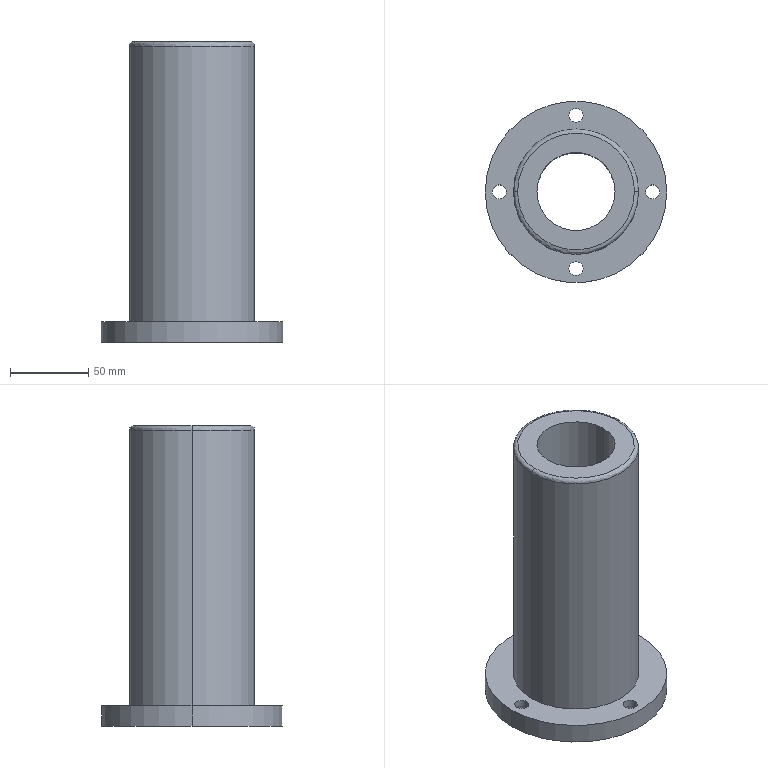Part | STEP file | LMG02-d50-Yiheda | 1 solid | 31 faces | box 116 x 116 x 192 mm | volume 653566 mm3 | cylinder 22 | plane 7 | spline 2 | commonest cylinder face diameters 9 x8 14 x8 50 x2 80 x2 116 x2
STEP:
#1=CARTESIAN_POINT('',(40.,0.,189.3));
#2=VERTEX_POINT('',#1);
#3=CARTESIAN_POINT('',(-40.,0.,189.3));
#4=VERTEX_POINT('',#3);
#5=CARTESIAN_POINT('',(0.,0.,189.3));
#6=DIRECTION('',(0.,0.,-1.));
#7=DIRECTION('',(-1.,0.,0.));
#8=AXIS2_PLACEMENT_3D('',#5,#6,#7);
#9=CIRCLE('',#8,40.);
#10=EDGE_CURVE('',#2,#4,#9,.T.);
#11=ORIENTED_EDGE('',*,*,#10,.F.);
#12=CARTESIAN_POINT('',(37.3,0.,192.));
#13=VERTEX_POINT('',#12);
#14=CARTESIAN_POINT('',(37.3,0.,189.3));
#15=DIRECTION('',(0.,-1.,0.));
#16=DIRECTION('',(1.,0.,0.));
#17=AXIS2_PLACEMENT_3D('',#14,#15,#16);
#18=CIRCLE('',#17,2.7);
#19=EDGE_CURVE('',#2,#13,#18,.T.);
#20=ORIENTED_EDGE('',*,*,#19,.T.);
#21=CARTESIAN_POINT('',(-37.3,0.,192.));
#22=VERTEX_POINT('',#21);
#23=CARTESIAN_POINT('',(37.3,0.,192.));
#24=CARTESIAN_POINT('',(37.3,-74.6,192.));
#25=CARTESIAN_POINT('',(-37.3,-74.6,192.));
#26=CARTESIAN_POINT('',(-37.3,0.,192.));
#27=(BOUNDED_CURVE()B_SPLINE_CURVE(3,(#23,#24,#25,#26),.UNSPECIFIED.,.F.,.T.)B_SPLINE_CURVE_WITH_KNOTS((4,4),(0.5,1.),.UNSPECIFIED.)CURVE()GEOMETRIC_REPRESENTATION_ITEM()RATIONAL_B_SPLINE_CURVE((1.,0.3333,0.3333,1.))REPRESENTATION_ITEM(''));
#28=EDGE_CURVE('',#13,#22,#27,.T.);
#29=ORIENTED_EDGE('',*,*,#28,.T.);
#30=CARTESIAN_POINT('',(-37.3,0.,189.3));
#31=DIRECTION('',(0.,1.,0.));
#32=DIRECTION('',(-1.,0.,0.));
#33=AXIS2_PLACEMENT_3D('',#30,#31,#32);
#34=CIRCLE('',#33,2.7);
#35=EDGE_CURVE('',#4,#22,#34,.T.);
#36=ORIENTED_EDGE('',*,*,#35,.F.);
#37=EDGE_LOOP('',(#11,#20,#29,#36));
#38=FACE_OUTER_BOUND('',#37,.T.);
#39=CARTESIAN_POINT('',(40.,0.,189.3));
#40=CARTESIAN_POINT('',(40.,-80.,189.3));
#41=CARTESIAN_POINT('',(-40.,-80.,189.3));
#42=CARTESIAN_POINT('',(-40.,0.,189.3));
#43=CARTESIAN_POINT('',(40.,0.,190.882));
#44=CARTESIAN_POINT('',(40.,-80.,190.882));
#45=CARTESIAN_POINT('',(-40.,-80.,190.882));
#46=CARTESIAN_POINT('',(-40.,0.,190.882));
#47=CARTESIAN_POINT('',(38.882,0.,192.));
#48=CARTESIAN_POINT('',(38.882,-77.763,192.));
#49=CARTESIAN_POINT('',(-38.882,-77.763,192.));
#50=CARTESIAN_POINT('',(-38.882,0.,192.));
#51=CARTESIAN_POINT('',(37.3,0.,192.));
#52=CARTESIAN_POINT('',(37.3,-74.6,192.));
#53=CARTESIAN_POINT('',(-37.3,-74.6,192.));
#54=CARTESIAN_POINT('',(-37.3,0.,192.));
#55=(BOUNDED_SURFACE()B_SPLINE_SURFACE(3,3,((#39,#40,#41,#42),(#43,#44,#45,#46),(#47,#48,#49,#50),(#51,#52,#53,#54)),.UNSPECIFIED.,.F.,.F.,.T.)B_SPLINE_SURFACE_WITH_KNOTS((4,4),(4,4),(0.,1.),(0.,1.),.UNSPECIFIED.)GEOMETRIC_REPRESENTATION_ITEM()RATIONAL_B_SPLINE_SURFACE(((1.,0.3333,0.3333,1.),(0.8047,0.2682,0.2682,0.8047),(0.8047,0.2682,0.2682,0.8047),(1.,0.3333,0.3333,1.)))REPRESENTATION_ITEM('')SURFACE());
#56=ADVANCED_FACE('',(#38),#55,.T.);
#57=CARTESIAN_POINT('',(0.,0.,189.3));
#58=DIRECTION('',(0.,0.,-1.));
#59=DIRECTION('',(-1.,0.,0.));
#60=AXIS2_PLACEMENT_3D('',#57,#58,#59);
#61=CIRCLE('',#60,40.);
#62=EDGE_CURVE('',#4,#2,#61,.T.);
#63=ORIENTED_EDGE('',*,*,#62,.T.);
#64=CARTESIAN_POINT('',(40.,0.,13.));
#65=VERTEX_POINT('',#64);
#66=CARTESIAN_POINT('',(40.,0.,0.));
#67=DIRECTION('',(0.,0.,-1.));
#68=VECTOR('',#67,1000.);
#69=LINE('',#66,#68);
#70=EDGE_CURVE('',#2,#65,#69,.T.);
#71=ORIENTED_EDGE('',*,*,#70,.T.);
#72=CARTESIAN_POINT('',(-40.,0.,13.));
#73=VERTEX_POINT('',#72);
#74=CARTESIAN_POINT('',(0.,0.,13.));
#75=DIRECTION('',(0.,0.,1.));
#76=DIRECTION('',(-1.,0.,0.));
#77=AXIS2_PLACEMENT_3D('',#74,#75,#76);
#78=CIRCLE('',#77,40.);
#79=EDGE_CURVE('',#65,#73,#78,.T.);
#80=ORIENTED_EDGE('',*,*,#79,.T.);
#81=CARTESIAN_POINT('',(-40.,0.,0.));
#82=DIRECTION('',(0.,0.,-1.));
#83=VECTOR('',#82,1000.);
#84=LINE('',#81,#83);
#85=EDGE_CURVE('',#4,#73,#84,.T.);
#86=ORIENTED_EDGE('',*,*,#85,.F.);
#87=EDGE_LOOP('',(#63,#71,#80,#86));
#88=FACE_OUTER_BOUND('',#87,.T.);
#89=CARTESIAN_POINT('',(0.,0.,0.));
#90=DIRECTION('',(0.,0.,-1.));
#91=DIRECTION('',(-1.,0.,0.));
#92=AXIS2_PLACEMENT_3D('',#89,#90,#91);
#93=CYLINDRICAL_SURFACE('',#92,40.);
#94=ADVANCED_FACE('',(#88),#93,.T.);
#95=CARTESIAN_POINT('',(58.,0.,13.));
#96=VERTEX_POINT('',#95);
#97=CARTESIAN_POINT('',(-58.,0.,13.));
#98=VERTEX_POINT('',#97);
#99=CARTESIAN_POINT('',(0.,0.,13.));
#100=DIRECTION('',(0.,0.,1.));
#101=DIRECTION('',(-1.,0.,0.));
#102=AXIS2_PLACEMENT_3D('',#99,#100,#101);
#103=CIRCLE('',#102,58.);
#104=EDGE_CURVE('',#96,#98,#103,.T.);
#105=ORIENTED_EDGE('',*,*,#104,.F.);
#106=CARTESIAN_POINT('',(58.,0.,0.));
#107=VERTEX_POINT('',#106);
#108=CARTESIAN_POINT('',(58.,0.,13.));
#109=DIRECTION('',(0.,0.,-1.));
#110=VECTOR('',#109,1000.);
#111=LINE('',#108,#110);
#112=EDGE_CURVE('',#96,#107,#111,.T.);
#113=ORIENTED_EDGE('',*,*,#112,.T.);
#114=CARTESIAN_POINT('',(-58.,0.,0.));
#115=VERTEX_POINT('',#114);
#116=CARTESIAN_POINT('',(0.,0.,0.));
#117=DIRECTION('',(0.,0.,1.));
#118=DIRECTION('',(-1.,0.,0.));
#119=AXIS2_PLACEMENT_3D('',#116,#117,#118);
#120=CIRCLE('',#119,58.);
#121=EDGE_CURVE('',#107,#115,#120,.T.);
#122=ORIENTED_EDGE('',*,*,#121,.T.);
#123=CARTESIAN_POINT('',(-58.,0.,13.));
#124=DIRECTION('',(0.,0.,-1.));
#125=VECTOR('',#124,1000.);
#126=LINE('',#123,#125);
#127=EDGE_CURVE('',#98,#115,#126,.T.);
#128=ORIENTED_EDGE('',*,*,#127,.F.);
#129=EDGE_LOOP('',(#105,#113,#122,#128));
#130=FACE_OUTER_BOUND('',#129,.T.);
#131=CARTESIAN_POINT('',(0.,0.,13.));
#132=DIRECTION('',(0.,0.,-1.));
#133=DIRECTION('',(-1.,0.,0.));
#134=AXIS2_PLACEMENT_3D('',#131,#132,#133);
#135=CYLINDRICAL_SURFACE('',#134,58.);
#136=ADVANCED_FACE('',(#130),#135,.T.);
#137=CARTESIAN_POINT('',(4.5,49.,13.));
#138=VERTEX_POINT('',#137);
#139=CARTESIAN_POINT('',(-4.5,49.,13.));
#140=VERTEX_POINT('',#139);
#141=CARTESIAN_POINT('',(0.,49.,13.));
#142=DIRECTION('',(0.,0.,-1.));
#143=DIRECTION('',(-1.,0.,0.));
#144=AXIS2_PLACEMENT_3D('',#141,#142,#143);
#145=CIRCLE('',#144,4.5);
#146=EDGE_CURVE('',#138,#140,#145,.T.);
#147=ORIENTED_EDGE('',*,*,#146,.F.);
#148=CARTESIAN_POINT('',(4.5,49.,8.1));
#149=VERTEX_POINT('',#148);
#150=CARTESIAN_POINT('',(4.5,49.,0.));
#151=DIRECTION('',(0.,0.,-1.));
#152=VECTOR('',#151,1000.);
#153=LINE('',#150,#152);
#154=EDGE_CURVE('',#138,#149,#153,.T.);
#155=ORIENTED_EDGE('',*,*,#154,.T.);
#156=CARTESIAN_POINT('',(-4.5,49.,8.1));
#157=VERTEX_POINT('',#156);
#158=CARTESIAN_POINT('',(0.,49.,8.1));
#159=DIRECTION('',(0.,0.,1.));
#160=DIRECTION('',(-1.,0.,0.));
#161=AXIS2_PLACEMENT_3D('',#158,#159,#160);
#162=CIRCLE('',#161,4.5);
#163=EDGE_CURVE('',#157,#149,#162,.T.);
#164=ORIENTED_EDGE('',*,*,#163,.F.);
#165=CARTESIAN_POINT('',(-4.5,49.,0.));
#166=DIRECTION('',(0.,0.,-1.));
#167=VECTOR('',#166,1000.);
#168=LINE('',#165,#167);
#169=EDGE_CURVE('',#140,#157,#168,.T.);
#170=ORIENTED_EDGE('',*,*,#169,.F.);
#171=EDGE_LOOP('',(#147,#155,#164,#170));
#172=FACE_OUTER_BOUND('',#171,.T.);
#173=CARTESIAN_POINT('',(0.,49.,0.));
#174=DIRECTION('',(0.,0.,-1.));
#175=DIRECTION('',(-1.,0.,0.));
#176=AXIS2_PLACEMENT_3D('',#173,#174,#175);
#177=CYLINDRICAL_SURFACE('',#176,4.5);
#178=ADVANCED_FACE('',(#172),#177,.F.);
#179=CARTESIAN_POINT('',(-4.5,-49.,8.1));
#180=VERTEX_POINT('',#179);
#181=CARTESIAN_POINT('',(4.5,-49.,8.1));
#182=VERTEX_POINT('',#181);
#183=CARTESIAN_POINT('',(0.,-49.,8.1));
#184=DIRECTION('',(0.,0.,1.));
#185=DIRECTION('',(1.,0.,0.));
#186=AXIS2_PLACEMENT_3D('',#183,#184,#185);
#187=CIRCLE('',#186,4.5);
#188=EDGE_CURVE('',#180,#182,#187,.T.);
#189=ORIENTED_EDGE('',*,*,#188,.F.);
#190=CARTESIAN_POINT('',(-4.5,-49.,13.));
#191=VERTEX_POINT('',#190);
#192=CARTESIAN_POINT('',(-4.5,-49.,13.));
#193=DIRECTION('',(0.,0.,1.));
#194=VECTOR('',#193,1000.);
#195=LINE('',#192,#194);
#196=EDGE_CURVE('',#180,#191,#195,.T.);
#197=ORIENTED_EDGE('',*,*,#196,.T.);
#198=CARTESIAN_POINT('',(4.5,-49.,13.));
#199=VERTEX_POINT('',#198);
#200=CARTESIAN_POINT('',(0.,-49.,13.));
#201=DIRECTION('',(0.,0.,-1.));
#202=DIRECTION('',(1.,0.,0.));
#203=AXIS2_PLACEMENT_3D('',#200,#201,#202);
#204=CIRCLE('',#203,4.5);
#205=EDGE_CURVE('',#199,#191,#204,.T.);
#206=ORIENTED_EDGE('',*,*,#205,.F.);
#207=CARTESIAN_POINT('',(4.5,-49.,13.));
#208=DIRECTION('',(0.,0.,1.));
#209=VECTOR('',#208,1000.);
#210=LINE('',#207,#209);
#211=EDGE_CURVE('',#182,#199,#210,.T.);
#212=ORIENTED_EDGE('',*,*,#211,.F.);
#213=EDGE_LOOP('',(#189,#197,#206,#212));
#214=FACE_OUTER_BOUND('',#213,.T.);
#215=CARTESIAN_POINT('',(0.,-49.,13.));
#216=DIRECTION('',(0.,0.,1.));
#217=DIRECTION('',(1.,0.,0.));
#218=AXIS2_PLACEMENT_3D('',#215,#216,#217);
#219=CYLINDRICAL_SURFACE('',#218,4.5);
#220=ADVANCED_FACE('',(#214),#219,.F.);
#221=CARTESIAN_POINT('',(-44.5,0.,13.));
#222=VERTEX_POINT('',#221);
#223=CARTESIAN_POINT('',(-53.5,0.,13.));
#224=VERTEX_POINT('',#223);
#225=CARTESIAN_POINT('',(-49.,0.,13.));
#226=DIRECTION('',(0.,0.,-1.));
#227=DIRECTION('',(-1.,0.,0.));
#228=AXIS2_PLACEMENT_3D('',#225,#226,#227);
#229=CIRCLE('',#228,4.5);
#230=EDGE_CURVE('',#222,#224,#229,.T.);
#231=ORIENTED_EDGE('',*,*,#230,.F.);
#232=CARTESIAN_POINT('',(-44.5,0.,8.1));
#233=VERTEX_POINT('',#232);
#234=CARTESIAN_POINT('',(-44.5,0.,0.));
#235=DIRECTION('',(0.,0.,-1.));
#236=VECTOR('',#235,1000.);
#237=LINE('',#234,#236);
#238=EDGE_CURVE('',#222,#233,#237,.T.);
#239=ORIENTED_EDGE('',*,*,#238,.T.);
#240=CARTESIAN_POINT('',(-53.5,0.,8.1));
#241=VERTEX_POINT('',#240);
#242=CARTESIAN_POINT('',(-49.,0.,8.1));
#243=DIRECTION('',(0.,0.,1.));
#244=DIRECTION('',(-1.,0.,0.));
#245=AXIS2_PLACEMENT_3D('',#242,#243,#244);
#246=CIRCLE('',#245,4.5);
#247=EDGE_CURVE('',#241,#233,#246,.T.);
#248=ORIENTED_EDGE('',*,*,#247,.F.);
#249=CARTESIAN_POINT('',(-53.5,0.,0.));
#250=DIRECTION('',(0.,0.,-1.));
#251=VECTOR('',#250,1000.);
#252=LINE('',#249,#251);
#253=EDGE_CURVE('',#224,#241,#252,.T.);
#254=ORIENTED_EDGE('',*,*,#253,.F.);
#255=EDGE_LOOP('',(#231,#239,#248,#254));
#256=FACE_OUTER_BOUND('',#255,.T.);
#257=CARTESIAN_POINT('',(-49.,0.,0.));
#258=DIRECTION('',(0.,0.,-1.));
#259=DIRECTION('',(-1.,0.,0.));
#260=AXIS2_PLACEMENT_3D('',#257,#258,#259);
#261=CYLINDRICAL_SURFACE('',#260,4.5);
#262=ADVANCED_FACE('',(#256),#261,.F.);
#263=CARTESIAN_POINT('',(44.5,0.,8.1));
#264=VERTEX_POINT('',#263);
#265=CARTESIAN_POINT('',(53.5,0.,8.1));
#266=VERTEX_POINT('',#265);
#267=CARTESIAN_POINT('',(49.,0.,8.1));
#268=DIRECTION('',(0.,0.,1.));
#269=DIRECTION('',(1.,0.,0.));
#270=AXIS2_PLACEMENT_3D('',#267,#268,#269);
#271=CIRCLE('',#270,4.5);
#272=EDGE_CURVE('',#264,#266,#271,.T.);
#273=ORIENTED_EDGE('',*,*,#272,.F.);
#274=CARTESIAN_POINT('',(44.5,0.,13.));
#275=VERTEX_POINT('',#274);
#276=CARTESIAN_POINT('',(44.5,0.,13.));
#277=DIRECTION('',(0.,0.,1.));
#278=VECTOR('',#277,1000.);
#279=LINE('',#276,#278);
#280=EDGE_CURVE('',#264,#275,#279,.T.);
#281=ORIENTED_EDGE('',*,*,#280,.T.);
#282=CARTESIAN_POINT('',(53.5,0.,13.));
#283=VERTEX_POINT('',#282);
#284=CARTESIAN_POINT('',(49.,0.,13.));
#285=DIRECTION('',(0.,0.,-1.));
#286=DIRECTION('',(1.,0.,0.));
#287=AXIS2_PLACEMENT_3D('',#284,#285,#286);
#288=CIRCLE('',#287,4.5);
#289=EDGE_CURVE('',#283,#275,#288,.T.);
#290=ORIENTED_EDGE('',*,*,#289,.F.);
#291=CARTESIAN_POINT('',(53.5,0.,13.));
#292=DIRECTION('',(0.,0.,1.));
#293=VECTOR('',#292,1000.);
#294=LINE('',#291,#293);
#295=EDGE_CURVE('',#266,#283,#294,.T.);
#296=ORIENTED_EDGE('',*,*,#295,.F.);
#297=EDGE_LOOP('',(#273,#281,#290,#296));
#298=FACE_OUTER_BOUND('',#297,.T.);
#299=CARTESIAN_POINT('',(49.,0.,13.));
#300=DIRECTION('',(0.,0.,1.));
#301=DIRECTION('',(1.,0.,0.));
#302=AXIS2_PLACEMENT_3D('',#299,#300,#301);
#303=CYLINDRICAL_SURFACE('',#302,4.5);
#304=ADVANCED_FACE('',(#298),#303,.F.);
#305=CARTESIAN_POINT('',(25.,0.,192.));
#306=VERTEX_POINT('',#305);
#307=CARTESIAN_POINT('',(-25.,0.,192.));
#308=VERTEX_POINT('',#307);
#309=CARTESIAN_POINT('',(0.,0.,192.));
#310=DIRECTION('',(0.,0.,-1.));
#311=DIRECTION('',(-1.,0.,0.));
#312=AXIS2_PLACEMENT_3D('',#309,#310,#311);
#313=CIRCLE('',#312,25.);
#314=EDGE_CURVE('',#306,#308,#313,.T.);
#315=ORIENTED_EDGE('',*,*,#314,.F.);
#316=CARTESIAN_POINT('',(25.,0.,0.));
#317=VERTEX_POINT('',#316);
#318=CARTESIAN_POINT('',(25.,0.,0.));
#319=DIRECTION('',(0.,0.,-1.));
#320=VECTOR('',#319,1000.);
#321=LINE('',#318,#320);
#322=EDGE_CURVE('',#306,#317,#321,.T.);
#323=ORIENTED_EDGE('',*,*,#322,.T.);
#324=CARTESIAN_POINT('',(-25.,0.,0.));
#325=VERTEX_POINT('',#324);
#326=CARTESIAN_POINT('',(0.,0.,0.));
#327=DIRECTION('',(0.,0.,1.));
#328=DIRECTION('',(-1.,0.,0.));
#329=AXIS2_PLACEMENT_3D('',#326,#327,#328);
#330=CIRCLE('',#329,25.);
#331=EDGE_CURVE('',#325,#317,#330,.T.);
#332=ORIENTED_EDGE('',*,*,#331,.F.);
#333=CARTESIAN_POINT('',(-25.,0.,0.));
#334=DIRECTION('',(0.,0.,-1.));
#335=VECTOR('',#334,1000.);
#336=LINE('',#333,#335);
#337=EDGE_CURVE('',#308,#325,#336,.T.);
#338=ORIENTED_EDGE('',*,*,#337,.F.);
#339=EDGE_LOOP('',(#315,#323,#332,#338));
#340=FACE_OUTER_BOUND('',#339,.T.);
#341=CARTESIAN_POINT('',(0.,0.,0.));
#342=DIRECTION('',(0.,0.,-1.));
#343=DIRECTION('',(-1.,0.,0.));
#344=AXIS2_PLACEMENT_3D('',#341,#342,#343);
#345=CYLINDRICAL_SURFACE('',#344,25.);
#346=ADVANCED_FACE('',(#340),#345,.F.);
#347=CARTESIAN_POINT('',(7.,49.,8.1));
#348=VERTEX_POINT('',#347);
#349=CARTESIAN_POINT('',(-7.,49.,8.1));
#350=VERTEX_POINT('',#349);
#351=CARTESIAN_POINT('',(0.,49.,8.1));
#352=DIRECTION('',(0.,0.,-1.));
#353=DIRECTION('',(-1.,0.,0.));
#354=AXIS2_PLACEMENT_3D('',#351,#352,#353);
#355=CIRCLE('',#354,7.);
#356=EDGE_CURVE('',#348,#350,#355,.T.);
#357=ORIENTED_EDGE('',*,*,#356,.F.);
#358=CARTESIAN_POINT('',(7.,49.,0.));
#359=VERTEX_POINT('',#358);
#360=CARTESIAN_POINT('',(7.,49.,0.));
#361=DIRECTION('',(0.,0.,-1.));
#362=VECTOR('',#361,1000.);
#363=LINE('',#360,#362);
#364=EDGE_CURVE('',#348,#359,#363,.T.);
#365=ORIENTED_EDGE('',*,*,#364,.T.);
#366=CARTESIAN_POINT('',(-7.,49.,0.));
#367=VERTEX_POINT('',#366);
#368=CARTESIAN_POINT('',(0.,49.,0.));
#369=DIRECTION('',(0.,0.,1.));
#370=DIRECTION('',(-1.,0.,0.));
#371=AXIS2_PLACEMENT_3D('',#368,#369,#370);
#372=CIRCLE('',#371,7.);
#373=EDGE_CURVE('',#367,#359,#372,.T.);
#374=ORIENTED_EDGE('',*,*,#373,.F.);
#375=CARTESIAN_POINT('',(-7.,49.,0.));
#376=DIRECTION('',(0.,0.,-1.));
#377=VECTOR('',#376,1000.);
#378=LINE('',#375,#377);
#379=EDGE_CURVE('',#350,#367,#378,.T.);
#380=ORIENTED_EDGE('',*,*,#379,.F.);
#381=EDGE_LOOP('',(#357,#365,#374,#380));
#382=FACE_OUTER_BOUND('',#381,.T.);
#383=CARTESIAN_POINT('',(0.,49.,0.));
#384=DIRECTION('',(0.,0.,-1.));
#385=DIRECTION('',(-1.,0.,0.));
#386=AXIS2_PLACEMENT_3D('',#383,#384,#385);
#387=CYLINDRICAL_SURFACE('',#386,7.);
#388=ADVANCED_FACE('',(#382),#387,.F.);
#389=CARTESIAN_POINT('',(-7.,-49.,0.));
#390=VERTEX_POINT('',#389);
#391=CARTESIAN_POINT('',(7.,-49.,0.));
#392=VERTEX_POINT('',#391);
#393=CARTESIAN_POINT('',(0.,-49.,0.));
#394=DIRECTION('',(0.,0.,1.));
#395=DIRECTION('',(1.,0.,0.));
#396=AXIS2_PLACEMENT_3D('',#393,#394,#395);
#397=CIRCLE('',#396,7.);
#398=EDGE_CURVE('',#390,#392,#397,.T.);
#399=ORIENTED_EDGE('',*,*,#398,.F.);
#400=CARTESIAN_POINT('',(-7.,-49.,8.1));
#401=VERTEX_POINT('',#400);
#402=CARTESIAN_POINT('',(-7.,-49.,13.));
#403=DIRECTION('',(0.,0.,1.));
#404=VECTOR('',#403,1000.);
#405=LINE('',#402,#404);
#406=EDGE_CURVE('',#390,#401,#405,.T.);
#407=ORIENTED_EDGE('',*,*,#406,.T.);
#408=CARTESIAN_POINT('',(7.,-49.,8.1));
#409=VERTEX_POINT('',#408);
#410=CARTESIAN_POINT('',(0.,-49.,8.1));
#411=DIRECTION('',(0.,0.,-1.));
#412=DIRECTION('',(1.,0.,0.));
#413=AXIS2_PLACEMENT_3D('',#410,#411,#412);
#414=CIRCLE('',#413,7.);
#415=EDGE_CURVE('',#409,#401,#414,.T.);
#416=ORIENTED_EDGE('',*,*,#415,.F.);
#417=CARTESIAN_POINT('',(7.,-49.,13.));
#418=DIRECTION('',(0.,0.,1.));
#419=VECTOR('',#418,1000.);
#420=LINE('',#417,#419);
#421=EDGE_CURVE('',#392,#409,#420,.T.);
#422=ORIENTED_EDGE('',*,*,#421,.F.);
#423=EDGE_LOOP('',(#399,#407,#416,#422));
#424=FACE_OUTER_BOUND('',#423,.T.);
#425=CARTESIAN_POINT('',(0.,-49.,13.));
#426=DIRECTION('',(0.,0.,1.));
#427=DIRECTION('',(1.,0.,0.));
#428=AXIS2_PLACEMENT_3D('',#425,#426,#427);
#429=CYLINDRICAL_SURFACE('',#428,7.);
#430=ADVANCED_FACE('',(#424),#429,.F.);
#431=CARTESIAN_POINT('',(-42.,0.,8.1));
#432=VERTEX_POINT('',#431);
#433=CARTESIAN_POINT('',(-56.,0.,8.1));
#434=VERTEX_POINT('',#433);
#435=CARTESIAN_POINT('',(-49.,0.,8.1));
#436=DIRECTION('',(0.,0.,-1.));
#437=DIRECTION('',(-1.,0.,0.));
#438=AXIS2_PLACEMENT_3D('',#435,#436,#437);
#439=CIRCLE('',#438,7.);
#440=EDGE_CURVE('',#432,#434,#439,.T.);
#441=ORIENTED_EDGE('',*,*,#440,.F.);
#442=CARTESIAN_POINT('',(-42.,0.,0.));
#443=VERTEX_POINT('',#442);
#444=CARTESIAN_POINT('',(-42.,0.,0.));
#445=DIRECTION('',(0.,0.,-1.));
#446=VECTOR('',#445,1000.);
#447=LINE('',#444,#446);
#448=EDGE_CURVE('',#432,#443,#447,.T.);
#449=ORIENTED_EDGE('',*,*,#448,.T.);
#450=CARTESIAN_POINT('',(-56.,0.,0.));
#451=VERTEX_POINT('',#450);
#452=CARTESIAN_POINT('',(-49.,0.,0.));
#453=DIRECTION('',(0.,0.,1.));
#454=DIRECTION('',(-1.,0.,0.));
#455=AXIS2_PLACEMENT_3D('',#452,#453,#454);
#456=CIRCLE('',#455,7.);
#457=EDGE_CURVE('',#451,#443,#456,.T.);
#458=ORIENTED_EDGE('',*,*,#457,.F.);
#459=CARTESIAN_POINT('',(-56.,0.,0.));
#460=DIRECTION('',(0.,0.,-1.));
#461=VECTOR('',#460,1000.);
#462=LINE('',#459,#461);
#463=EDGE_CURVE('',#434,#451,#462,.T.);
#464=ORIENTED_EDGE('',*,*,#463,.F.);
#465=EDGE_LOOP('',(#441,#449,#458,#464));
#466=FACE_OUTER_BOUND('',#465,.T.);
#467=CARTESIAN_POINT('',(-49.,0.,0.));
#468=DIRECTION('',(0.,0.,-1.));
#469=DIRECTION('',(-1.,0.,0.));
#470=AXIS2_PLACEMENT_3D('',#467,#468,#469);
#471=CYLINDRICAL_SURFACE('',#470,7.);
#472=ADVANCED_FACE('',(#466),#471,.F.);
#473=CARTESIAN_POINT('',(42.,0.,0.));
#474=VERTEX_POINT('',#473);
#475=CARTESIAN_POINT('',(56.,0.,0.));
#476=VERTEX_POINT('',#475);
#477=CARTESIAN_POINT('',(49.,0.,0.));
#478=DIRECTION('',(0.,0.,1.));
#479=DIRECTION('',(1.,0.,0.));
#480=AXIS2_PLACEMENT_3D('',#477,#478,#479);
#481=CIRCLE('',#480,7.);
#482=EDGE_CURVE('',#474,#476,#481,.T.);
#483=ORIENTED_EDGE('',*,*,#482,.F.);
#484=CARTESIAN_POINT('',(42.,0.,8.1));
#485=VERTEX_POINT('',#484);
#486=CARTESIAN_POINT('',(42.,0.,13.));
#487=DIRECTION('',(0.,0.,1.));
#488=VECTOR('',#487,1000.);
#489=LINE('',#486,#488);
#490=EDGE_CURVE('',#474,#485,#489,.T.);
#491=ORIENTED_EDGE('',*,*,#490,.T.);
#492=CARTESIAN_POINT('',(56.,0.,8.1));
#493=VERTEX_POINT('',#492);
#494=CARTESIAN_POINT('',(49.,0.,8.1));
#495=DIRECTION('',(0.,0.,-1.));
#496=DIRECTION('',(1.,0.,0.));
#497=AXIS2_PLACEMENT_3D('',#494,#495,#496);
#498=CIRCLE('',#497,7.);
#499=EDGE_CURVE('',#493,#485,#498,.T.);
#500=ORIENTED_EDGE('',*,*,#499,.F.);
#501=CARTESIAN_POINT('',(56.,0.,13.));
#502=DIRECTION('',(0.,0.,1.));
#503=VECTOR('',#502,1000.);
#504=LINE('',#501,#503);
#505=EDGE_CURVE('',#476,#493,#504,.T.);
#506=ORIENTED_EDGE('',*,*,#505,.F.);
#507=EDGE_LOOP('',(#483,#491,#500,#506));
#508=FACE_OUTER_BOUND('',#507,.T.);
#509=CARTESIAN_POINT('',(49.,0.,13.));
#510=DIRECTION('',(0.,0.,1.));
#511=DIRECTION('',(1.,0.,0.));
#512=AXIS2_PLACEMENT_3D('',#509,#510,#511);
#513=CYLINDRICAL_SURFACE('',#512,7.);
#514=ADVANCED_FACE('',(#508),#513,.F.);
#515=ORIENTED_EDGE('',*,*,#70,.F.);
#516=ORIENTED_EDGE('',*,*,#10,.T.);
#517=ORIENTED_EDGE('',*,*,#85,.T.);
#518=CARTESIAN_POINT('',(0.,0.,13.));
#519=DIRECTION('',(0.,0.,1.));
#520=DIRECTION('',(-1.,0.,0.));
#521=AXIS2_PLACEMENT_3D('',#518,#519,#520);
#522=CIRCLE('',#521,40.);
#523=EDGE_CURVE('',#73,#65,#522,.T.);
#524=ORIENTED_EDGE('',*,*,#523,.T.);
#525=EDGE_LOOP('',(#515,#516,#517,#524));
#526=FACE_OUTER_BOUND('',#525,.T.);
#527=CARTESIAN_POINT('',(0.,0.,0.));
#528=DIRECTION('',(0.,0.,-1.));
#529=DIRECTION('',(-1.,0.,0.));
#530=AXIS2_PLACEMENT_3D('',#527,#528,#529);
#531=CYLINDRICAL_SURFACE('',#530,40.);
#532=ADVANCED_FACE('',(#526),#531,.T.);
#533=CARTESIAN_POINT('',(0.,0.,13.));
#534=DIRECTION('',(0.,0.,1.));
#535=DIRECTION('',(-1.,0.,0.));
#536=AXIS2_PLACEMENT_3D('',#533,#534,#535);
#537=CIRCLE('',#536,58.);
#538=EDGE_CURVE('',#98,#96,#537,.T.);
#539=ORIENTED_EDGE('',*,*,#538,.T.);
#540=ORIENTED_EDGE('',*,*,#104,.T.);
#541=EDGE_LOOP('',(#539,#540));
#542=FACE_OUTER_BOUND('',#541,.T.);
#543=ORIENTED_EDGE('',*,*,#523,.F.);
#544=ORIENTED_EDGE('',*,*,#79,.F.);
#545=EDGE_LOOP('',(#543,#544));
#546=FACE_BOUND('',#545,.T.);
#547=CARTESIAN_POINT('',(0.,49.,13.));
#548=DIRECTION('',(0.,0.,-1.));
#549=DIRECTION('',(-1.,0.,0.));
#550=AXIS2_PLACEMENT_3D('',#547,#548,#549);
#551=CIRCLE('',#550,4.5);
#552=EDGE_CURVE('',#140,#138,#551,.T.);
#553=ORIENTED_EDGE('',*,*,#552,.T.);
#554=ORIENTED_EDGE('',*,*,#146,.T.);
#555=EDGE_LOOP('',(#553,#554));
#556=FACE_BOUND('',#555,.T.);
#557=ORIENTED_EDGE('',*,*,#205,.T.);
#558=CARTESIAN_POINT('',(0.,-49.,13.));
#559=DIRECTION('',(0.,0.,-1.));
#560=DIRECTION('',(1.,0.,0.));
#561=AXIS2_PLACEMENT_3D('',#558,#559,#560);
#562=CIRCLE('',#561,4.5);
#563=EDGE_CURVE('',#191,#199,#562,.T.);
#564=ORIENTED_EDGE('',*,*,#563,.T.);
#565=EDGE_LOOP('',(#557,#564));
#566=FACE_BOUND('',#565,.T.);
#567=CARTESIAN_POINT('',(-49.,0.,13.));
#568=DIRECTION('',(0.,0.,-1.));
#569=DIRECTION('',(-1.,0.,0.));
#570=AXIS2_PLACEMENT_3D('',#567,#568,#569);
#571=CIRCLE('',#570,4.5);
#572=EDGE_CURVE('',#224,#222,#571,.T.);
#573=ORIENTED_EDGE('',*,*,#572,.T.);
#574=ORIENTED_EDGE('',*,*,#230,.T.);
#575=EDGE_LOOP('',(#573,#574));
#576=FACE_BOUND('',#575,.T.);
#577=ORIENTED_EDGE('',*,*,#289,.T.);
#578=CARTESIAN_POINT('',(49.,0.,13.));
#579=DIRECTION('',(0.,0.,-1.));
#580=DIRECTION('',(1.,0.,0.));
#581=AXIS2_PLACEMENT_3D('',#578,#579,#580);
#582=CIRCLE('',#581,4.5);
#583=EDGE_CURVE('',#275,#283,#582,.T.);
#584=ORIENTED_EDGE('',*,*,#583,.T.);
#585=EDGE_LOOP('',(#577,#584));
#586=FACE_BOUND('',#585,.T.);
#587=CARTESIAN_POINT('',(0.,0.,13.));
#588=DIRECTION('',(0.,0.,1.));
#589=DIRECTION('',(1.,0.,0.));
#590=AXIS2_PLACEMENT_3D('',#587,#588,#589);
#591=PLANE('',#590);
#592=ADVANCED_FACE('',(#542,#546,#556,#566,#576,#586),#591,.T.);
#593=ORIENTED_EDGE('',*,*,#19,.F.);
#594=ORIENTED_EDGE('',*,*,#62,.F.);
#595=ORIENTED_EDGE('',*,*,#35,.T.);
#596=CARTESIAN_POINT('',(-37.3,0.,192.));
#597=CARTESIAN_POINT('',(-37.3,74.6,192.));
#598=CARTESIAN_POINT('',(37.3,74.6,192.));
#599=CARTESIAN_POINT('',(37.3,0.,192.));
#600=(BOUNDED_CURVE()B_SPLINE_CURVE(3,(#596,#597,#598,#599),.UNSPECIFIED.,.F.,.F.)B_SPLINE_CURVE_WITH_KNOTS((4,4),(0.,0.5),.UNSPECIFIED.)CURVE()GEOMETRIC_REPRESENTATION_ITEM()RATIONAL_B_SPLINE_CURVE((1.,0.3333,0.3333,1.))REPRESENTATION_ITEM(''));
#601=EDGE_CURVE('',#22,#13,#600,.T.);
#602=ORIENTED_EDGE('',*,*,#601,.T.);
#603=EDGE_LOOP('',(#593,#594,#595,#602));
#604=FACE_OUTER_BOUND('',#603,.T.);
#605=CARTESIAN_POINT('',(-40.,0.,189.3));
#606=CARTESIAN_POINT('',(-40.,80.,189.3));
#607=CARTESIAN_POINT('',(40.,80.,189.3));
#608=CARTESIAN_POINT('',(40.,0.,189.3));
#609=CARTESIAN_POINT('',(-40.,0.,190.882));
#610=CARTESIAN_POINT('',(-40.,80.,190.882));
#611=CARTESIAN_POINT('',(40.,80.,190.882));
#612=CARTESIAN_POINT('',(40.,0.,190.882));
#613=CARTESIAN_POINT('',(-38.882,0.,192.));
#614=CARTESIAN_POINT('',(-38.882,77.763,192.));
#615=CARTESIAN_POINT('',(38.882,77.763,192.));
#616=CARTESIAN_POINT('',(38.882,0.,192.));
#617=CARTESIAN_POINT('',(-37.3,0.,192.));
#618=CARTESIAN_POINT('',(-37.3,74.6,192.));
#619=CARTESIAN_POINT('',(37.3,74.6,192.));
#620=CARTESIAN_POINT('',(37.3,0.,192.));
#621=(BOUNDED_SURFACE()B_SPLINE_SURFACE(3,3,((#605,#606,#607,#608),(#609,#610,#611,#612),(#613,#614,#615,#616),(#617,#618,#619,#620)),.UNSPECIFIED.,.F.,.F.,.T.)B_SPLINE_SURFACE_WITH_KNOTS((4,4),(4,4),(0.,1.),(0.,1.),.UNSPECIFIED.)GEOMETRIC_REPRESENTATION_ITEM()RATIONAL_B_SPLINE_SURFACE(((1.,0.3333,0.3333,1.),(0.8047,0.2682,0.2682,0.8047),(0.8047,0.2682,0.2682,0.8047),(1.,0.3333,0.3333,1.)))REPRESENTATION_ITEM('')SURFACE());
#622=ADVANCED_FACE('',(#604),#621,.T.);
#623=ORIENTED_EDGE('',*,*,#112,.F.);
#624=ORIENTED_EDGE('',*,*,#538,.F.);
#625=ORIENTED_EDGE('',*,*,#127,.T.);
#626=CARTESIAN_POINT('',(0.,0.,0.));
#627=DIRECTION('',(0.,0.,1.));
#628=DIRECTION('',(-1.,0.,0.));
#629=AXIS2_PLACEMENT_3D('',#626,#627,#628);
#630=CIRCLE('',#629,58.);
#631=EDGE_CURVE('',#115,#107,#630,.T.);
#632=ORIENTED_EDGE('',*,*,#631,.T.);
#633=EDGE_LOOP('',(#623,#624,#625,#632));
#634=FACE_OUTER_BOUND('',#633,.T.);
#635=CARTESIAN_POINT('',(0.,0.,13.));
#636=DIRECTION('',(0.,0.,-1.));
#637=DIRECTION('',(-1.,0.,0.));
#638=AXIS2_PLACEMENT_3D('',#635,#636,#637);
#639=CYLINDRICAL_SURFACE('',#638,58.);
#640=ADVANCED_FACE('',(#634),#639,.T.);
#641=ORIENTED_EDGE('',*,*,#154,.F.);
#642=ORIENTED_EDGE('',*,*,#552,.F.);
#643=ORIENTED_EDGE('',*,*,#169,.T.);
#644=CARTESIAN_POINT('',(0.,49.,8.1));
#645=DIRECTION('',(0.,0.,1.));
#646=DIRECTION('',(-1.,0.,0.));
#647=AXIS2_PLACEMENT_3D('',#644,#645,#646);
#648=CIRCLE('',#647,4.5);
#649=EDGE_CURVE('',#149,#157,#648,.T.);
#650=ORIENTED_EDGE('',*,*,#649,.F.);
#651=EDGE_LOOP('',(#641,#642,#643,#650));
#652=FACE_OUTER_BOUND('',#651,.T.);
#653=CARTESIAN_POINT('',(0.,49.,0.));
#654=DIRECTION('',(0.,0.,-1.));
#655=DIRECTION('',(-1.,0.,0.));
#656=AXIS2_PLACEMENT_3D('',#653,#654,#655);
#657=CYLINDRICAL_SURFACE('',#656,4.5);
#658=ADVANCED_FACE('',(#652),#657,.F.);
#659=ORIENTED_EDGE('',*,*,#196,.F.);
#660=CARTESIAN_POINT('',(0.,-49.,8.1));
#661=DIRECTION('',(0.,0.,1.));
#662=DIRECTION('',(1.,0.,0.));
#663=AXIS2_PLACEMENT_3D('',#660,#661,#662);
#664=CIRCLE('',#663,4.5);
#665=EDGE_CURVE('',#182,#180,#664,.T.);
#666=ORIENTED_EDGE('',*,*,#665,.F.);
#667=ORIENTED_EDGE('',*,*,#211,.T.);
#668=ORIENTED_EDGE('',*,*,#563,.F.);
#669=EDGE_LOOP('',(#659,#666,#667,#668));
#670=FACE_OUTER_BOUND('',#669,.T.);
#671=CARTESIAN_POINT('',(0.,-49.,13.));
#672=DIRECTION('',(0.,0.,1.));
#673=DIRECTION('',(1.,0.,0.));
#674=AXIS2_PLACEMENT_3D('',#671,#672,#673);
#675=CYLINDRICAL_SURFACE('',#674,4.5);
#676=ADVANCED_FACE('',(#670),#675,.F.);
#677=ORIENTED_EDGE('',*,*,#238,.F.);
#678=ORIENTED_EDGE('',*,*,#572,.F.);
#679=ORIENTED_EDGE('',*,*,#253,.T.);
#680=CARTESIAN_POINT('',(-49.,0.,8.1));
#681=DIRECTION('',(0.,0.,1.));
#682=DIRECTION('',(-1.,0.,0.));
#683=AXIS2_PLACEMENT_3D('',#680,#681,#682);
#684=CIRCLE('',#683,4.5);
#685=EDGE_CURVE('',#233,#241,#684,.T.);
#686=ORIENTED_EDGE('',*,*,#685,.F.);
#687=EDGE_LOOP('',(#677,#678,#679,#686));
#688=FACE_OUTER_BOUND('',#687,.T.);
#689=CARTESIAN_POINT('',(-49.,0.,0.));
#690=DIRECTION('',(0.,0.,-1.));
#691=DIRECTION('',(-1.,0.,0.));
#692=AXIS2_PLACEMENT_3D('',#689,#690,#691);
#693=CYLINDRICAL_SURFACE('',#692,4.5);
#694=ADVANCED_FACE('',(#688),#693,.F.);
#695=ORIENTED_EDGE('',*,*,#280,.F.);
#696=CARTESIAN_POINT('',(49.,0.,8.1));
#697=DIRECTION('',(0.,0.,1.));
#698=DIRECTION('',(1.,0.,0.));
#699=AXIS2_PLACEMENT_3D('',#696,#697,#698);
#700=CIRCLE('',#699,4.5);
#701=EDGE_CURVE('',#266,#264,#700,.T.);
#702=ORIENTED_EDGE('',*,*,#701,.F.);
#703=ORIENTED_EDGE('',*,*,#295,.T.);
#704=ORIENTED_EDGE('',*,*,#583,.F.);
#705=EDGE_LOOP('',(#695,#702,#703,#704));
#706=FACE_OUTER_BOUND('',#705,.T.);
#707=CARTESIAN_POINT('',(49.,0.,13.));
#708=DIRECTION('',(0.,0.,1.));
#709=DIRECTION('',(1.,0.,0.));
#710=AXIS2_PLACEMENT_3D('',#707,#708,#709);
#711=CYLINDRICAL_SURFACE('',#710,4.5);
#712=ADVANCED_FACE('',(#706),#711,.F.);
#713=ORIENTED_EDGE('',*,*,#601,.F.);
#714=ORIENTED_EDGE('',*,*,#28,.F.);
#715=EDGE_LOOP('',(#713,#714));
#716=FACE_OUTER_BOUND('',#715,.T.);
#717=CARTESIAN_POINT('',(0.,0.,192.));
#718=DIRECTION('',(0.,0.,-1.));
#719=DIRECTION('',(-1.,0.,0.));
#720=AXIS2_PLACEMENT_3D('',#717,#718,#719);
#721=CIRCLE('',#720,25.);
#722=EDGE_CURVE('',#308,#306,#721,.T.);
#723=ORIENTED_EDGE('',*,*,#722,.T.);
#724=ORIENTED_EDGE('',*,*,#314,.T.);
#725=EDGE_LOOP('',(#723,#724));
#726=FACE_BOUND('',#725,.T.);
#727=CARTESIAN_POINT('',(0.,37.3,192.));
#728=DIRECTION('',(0.,0.,1.));
#729=DIRECTION('',(1.,0.,0.));
#730=AXIS2_PLACEMENT_3D('',#727,#728,#729);
#731=PLANE('',#730);
#732=ADVANCED_FACE('',(#716,#726),#731,.T.);
#733=ORIENTED_EDGE('',*,*,#631,.F.);
#734=ORIENTED_EDGE('',*,*,#121,.F.);
#735=EDGE_LOOP('',(#733,#734));
#736=FACE_OUTER_BOUND('',#735,.T.);
#737=ORIENTED_EDGE('',*,*,#331,.T.);
#738=CARTESIAN_POINT('',(0.,0.,0.));
#739=DIRECTION('',(0.,0.,1.));
#740=DIRECTION('',(-1.,0.,0.));
#741=AXIS2_PLACEMENT_3D('',#738,#739,#740);
#742=CIRCLE('',#741,25.);
#743=EDGE_CURVE('',#317,#325,#742,.T.);
#744=ORIENTED_EDGE('',*,*,#743,.T.);
#745=EDGE_LOOP('',(#737,#744));
#746=FACE_BOUND('',#745,.T.);
#747=ORIENTED_EDGE('',*,*,#373,.T.);
#748=CARTESIAN_POINT('',(0.,49.,0.));
#749=DIRECTION('',(0.,0.,1.));
#750=DIRECTION('',(-1.,0.,0.));
#751=AXIS2_PLACEMENT_3D('',#748,#749,#750);
#752=CIRCLE('',#751,7.);
#753=EDGE_CURVE('',#359,#367,#752,.T.);
#754=ORIENTED_EDGE('',*,*,#753,.T.);
#755=EDGE_LOOP('',(#747,#754));
#756=FACE_BOUND('',#755,.T.);
#757=CARTESIAN_POINT('',(0.,-49.,0.));
#758=DIRECTION('',(0.,0.,1.));
#759=DIRECTION('',(1.,0.,0.));
#760=AXIS2_PLACEMENT_3D('',#757,#758,#759);
#761=CIRCLE('',#760,7.);
#762=EDGE_CURVE('',#392,#390,#761,.T.);
#763=ORIENTED_EDGE('',*,*,#762,.T.);
#764=ORIENTED_EDGE('',*,*,#398,.T.);
#765=EDGE_LOOP('',(#763,#764));
#766=FACE_BOUND('',#765,.T.);
#767=ORIENTED_EDGE('',*,*,#457,.T.);
#768=CARTESIAN_POINT('',(-49.,0.,0.));
#769=DIRECTION('',(0.,0.,1.));
#770=DIRECTION('',(-1.,0.,0.));
#771=AXIS2_PLACEMENT_3D('',#768,#769,#770);
#772=CIRCLE('',#771,7.);
#773=EDGE_CURVE('',#443,#451,#772,.T.);
#774=ORIENTED_EDGE('',*,*,#773,.T.);
#775=EDGE_LOOP('',(#767,#774));
#776=FACE_BOUND('',#775,.T.);
#777=CARTESIAN_POINT('',(49.,0.,0.));
#778=DIRECTION('',(0.,0.,1.));
#779=DIRECTION('',(1.,0.,0.));
#780=AXIS2_PLACEMENT_3D('',#777,#778,#779);
#781=CIRCLE('',#780,7.);
#782=EDGE_CURVE('',#476,#474,#781,.T.);
#783=ORIENTED_EDGE('',*,*,#782,.T.);
#784=ORIENTED_EDGE('',*,*,#482,.T.);
#785=EDGE_LOOP('',(#783,#784));
#786=FACE_BOUND('',#785,.T.);
#787=CARTESIAN_POINT('',(0.,25.,0.));
#788=DIRECTION('',(0.,0.,-1.));
#789=DIRECTION('',(-1.,0.,0.));
#790=AXIS2_PLACEMENT_3D('',#787,#788,#789);
#791=PLANE('',#790);
#792=ADVANCED_FACE('',(#736,#746,#756,#766,#776,#786),#791,.T.);
#793=ORIENTED_EDGE('',*,*,#163,.T.);
#794=ORIENTED_EDGE('',*,*,#649,.T.);
#795=EDGE_LOOP('',(#793,#794));
#796=FACE_BOUND('',#795,.T.);
#797=CARTESIAN_POINT('',(0.,49.,8.1));
#798=DIRECTION('',(0.,0.,-1.));
#799=DIRECTION('',(-1.,0.,0.));
#800=AXIS2_PLACEMENT_3D('',#797,#798,#799);
#801=CIRCLE('',#800,7.);
#802=EDGE_CURVE('',#350,#348,#801,.T.);
#803=ORIENTED_EDGE('',*,*,#802,.T.);
#804=ORIENTED_EDGE('',*,*,#356,.T.);
#805=EDGE_LOOP('',(#803,#804));
#806=FACE_OUTER_BOUND('',#805,.T.);
#807=CARTESIAN_POINT('',(0.,53.5,8.1));
#808=DIRECTION('',(0.,0.,-1.));
#809=DIRECTION('',(-1.,0.,0.));
#810=AXIS2_PLACEMENT_3D('',#807,#808,#809);
#811=PLANE('',#810);
#812=ADVANCED_FACE('',(#796,#806),#811,.T.);
#813=ORIENTED_EDGE('',*,*,#415,.T.);
#814=CARTESIAN_POINT('',(0.,-49.,8.1));
#815=DIRECTION('',(0.,0.,-1.));
#816=DIRECTION('',(1.,0.,0.));
#817=AXIS2_PLACEMENT_3D('',#814,#815,#816);
#818=CIRCLE('',#817,7.);
#819=EDGE_CURVE('',#401,#409,#818,.T.);
#820=ORIENTED_EDGE('',*,*,#819,.T.);
#821=EDGE_LOOP('',(#813,#820));
#822=FACE_OUTER_BOUND('',#821,.T.);
#823=ORIENTED_EDGE('',*,*,#665,.T.);
#824=ORIENTED_EDGE('',*,*,#188,.T.);
#825=EDGE_LOOP('',(#823,#824));
#826=FACE_BOUND('',#825,.T.);
#827=CARTESIAN_POINT('',(0.,-56.,8.1));
#828=DIRECTION('',(0.,0.,-1.));
#829=DIRECTION('',(-1.,0.,0.));
#830=AXIS2_PLACEMENT_3D('',#827,#828,#829);
#831=PLANE('',#830);
#832=ADVANCED_FACE('',(#822,#826),#831,.T.);
#833=ORIENTED_EDGE('',*,*,#247,.T.);
#834=ORIENTED_EDGE('',*,*,#685,.T.);
#835=EDGE_LOOP('',(#833,#834));
#836=FACE_BOUND('',#835,.T.);
#837=CARTESIAN_POINT('',(-49.,0.,8.1));
#838=DIRECTION('',(0.,0.,-1.));
#839=DIRECTION('',(-1.,0.,0.));
#840=AXIS2_PLACEMENT_3D('',#837,#838,#839);
#841=CIRCLE('',#840,7.);
#842=EDGE_CURVE('',#434,#432,#841,.T.);
#843=ORIENTED_EDGE('',*,*,#842,.T.);
#844=ORIENTED_EDGE('',*,*,#440,.T.);
#845=EDGE_LOOP('',(#843,#844));
#846=FACE_OUTER_BOUND('',#845,.T.);
#847=CARTESIAN_POINT('',(-53.5,0.,8.1));
#848=DIRECTION('',(0.,0.,-1.));
#849=DIRECTION('',(-1.,0.,0.));
#850=AXIS2_PLACEMENT_3D('',#847,#848,#849);
#851=PLANE('',#850);
#852=ADVANCED_FACE('',(#836,#846),#851,.T.);
#853=ORIENTED_EDGE('',*,*,#499,.T.);
#854=CARTESIAN_POINT('',(49.,0.,8.1));
#855=DIRECTION('',(0.,0.,-1.));
#856=DIRECTION('',(1.,0.,0.));
#857=AXIS2_PLACEMENT_3D('',#854,#855,#856);
#858=CIRCLE('',#857,7.);
#859=EDGE_CURVE('',#485,#493,#858,.T.);
#860=ORIENTED_EDGE('',*,*,#859,.T.);
#861=EDGE_LOOP('',(#853,#860));
#862=FACE_OUTER_BOUND('',#861,.T.);
#863=ORIENTED_EDGE('',*,*,#701,.T.);
#864=ORIENTED_EDGE('',*,*,#272,.T.);
#865=EDGE_LOOP('',(#863,#864));
#866=FACE_BOUND('',#865,.T.);
#867=CARTESIAN_POINT('',(56.,0.,8.1));
#868=DIRECTION('',(0.,0.,-1.));
#869=DIRECTION('',(-1.,0.,0.));
#870=AXIS2_PLACEMENT_3D('',#867,#868,#869);
#871=PLANE('',#870);
#872=ADVANCED_FACE('',(#862,#866),#871,.T.);
#873=ORIENTED_EDGE('',*,*,#322,.F.);
#874=ORIENTED_EDGE('',*,*,#722,.F.);
#875=ORIENTED_EDGE('',*,*,#337,.T.);
#876=ORIENTED_EDGE('',*,*,#743,.F.);
#877=EDGE_LOOP('',(#873,#874,#875,#876));
#878=FACE_OUTER_BOUND('',#877,.T.);
#879=CARTESIAN_POINT('',(0.,0.,0.));
#880=DIRECTION('',(0.,0.,-1.));
#881=DIRECTION('',(-1.,0.,0.));
#882=AXIS2_PLACEMENT_3D('',#879,#880,#881);
#883=CYLINDRICAL_SURFACE('',#882,25.);
#884=ADVANCED_FACE('',(#878),#883,.F.);
#885=ORIENTED_EDGE('',*,*,#364,.F.);
#886=ORIENTED_EDGE('',*,*,#802,.F.);
#887=ORIENTED_EDGE('',*,*,#379,.T.);
#888=ORIENTED_EDGE('',*,*,#753,.F.);
#889=EDGE_LOOP('',(#885,#886,#887,#888));
#890=FACE_OUTER_BOUND('',#889,.T.);
#891=CARTESIAN_POINT('',(0.,49.,0.));
#892=DIRECTION('',(0.,0.,-1.));
#893=DIRECTION('',(-1.,0.,0.));
#894=AXIS2_PLACEMENT_3D('',#891,#892,#893);
#895=CYLINDRICAL_SURFACE('',#894,7.);
#896=ADVANCED_FACE('',(#890),#895,.F.);
#897=ORIENTED_EDGE('',*,*,#406,.F.);
#898=ORIENTED_EDGE('',*,*,#762,.F.);
#899=ORIENTED_EDGE('',*,*,#421,.T.);
#900=ORIENTED_EDGE('',*,*,#819,.F.);
#901=EDGE_LOOP('',(#897,#898,#899,#900));
#902=FACE_OUTER_BOUND('',#901,.T.);
#903=CARTESIAN_POINT('',(0.,-49.,13.));
#904=DIRECTION('',(0.,0.,1.));
#905=DIRECTION('',(1.,0.,0.));
#906=AXIS2_PLACEMENT_3D('',#903,#904,#905);
#907=CYLINDRICAL_SURFACE('',#906,7.);
#908=ADVANCED_FACE('',(#902),#907,.F.);
#909=ORIENTED_EDGE('',*,*,#448,.F.);
#910=ORIENTED_EDGE('',*,*,#842,.F.);
#911=ORIENTED_EDGE('',*,*,#463,.T.);
#912=ORIENTED_EDGE('',*,*,#773,.F.);
#913=EDGE_LOOP('',(#909,#910,#911,#912));
#914=FACE_OUTER_BOUND('',#913,.T.);
#915=CARTESIAN_POINT('',(-49.,0.,0.));
#916=DIRECTION('',(0.,0.,-1.));
#917=DIRECTION('',(-1.,0.,0.));
#918=AXIS2_PLACEMENT_3D('',#915,#916,#917);
#919=CYLINDRICAL_SURFACE('',#918,7.);
#920=ADVANCED_FACE('',(#914),#919,.F.);
#921=ORIENTED_EDGE('',*,*,#490,.F.);
#922=ORIENTED_EDGE('',*,*,#782,.F.);
#923=ORIENTED_EDGE('',*,*,#505,.T.);
#924=ORIENTED_EDGE('',*,*,#859,.F.);
#925=EDGE_LOOP('',(#921,#922,#923,#924));
#926=FACE_OUTER_BOUND('',#925,.T.);
#927=CARTESIAN_POINT('',(49.,0.,13.));
#928=DIRECTION('',(0.,0.,1.));
#929=DIRECTION('',(1.,0.,0.));
#930=AXIS2_PLACEMENT_3D('',#927,#928,#929);
#931=CYLINDRICAL_SURFACE('',#930,7.);
#932=ADVANCED_FACE('',(#926),#931,.F.);
#933=CLOSED_SHELL('',(#56,#94,#136,#178,#220,#262,#304,#346,#388,#430,#472,#514,#532,#592,#622,#640,#658,#676,#694,#712,#732,#792,#812,#832,#852,#872,#884,#896,#908,#920,#932));
#934=MANIFOLD_SOLID_BREP('',#933);
#935=CARTESIAN_POINT('',(0.,0.,0.));
#936=DIRECTION('',(0.,0.,1.));
#937=DIRECTION('',(1.,0.,0.));
#938=AXIS2_PLACEMENT_3D('',#935,#936,#937);
#939=(LENGTH_UNIT()NAMED_UNIT(*)SI_UNIT(.MILLI.,.METRE.));
#940=UNCERTAINTY_MEASURE_WITH_UNIT(LENGTH_MEASURE(0.00001),#939,'','');
#941=(NAMED_UNIT(*)PLANE_ANGLE_UNIT()SI_UNIT($,.RADIAN.));
#942=(NAMED_UNIT(*)SI_UNIT($,.STERADIAN.)SOLID_ANGLE_UNIT());
#943=(GEOMETRIC_REPRESENTATION_CONTEXT(3)GLOBAL_UNCERTAINTY_ASSIGNED_CONTEXT((#940))GLOBAL_UNIT_ASSIGNED_CONTEXT((#939,#941,#942))REPRESENTATION_CONTEXT('',''));
#944=ADVANCED_BREP_SHAPE_REPRESENTATION('',(#934,#938),#943);